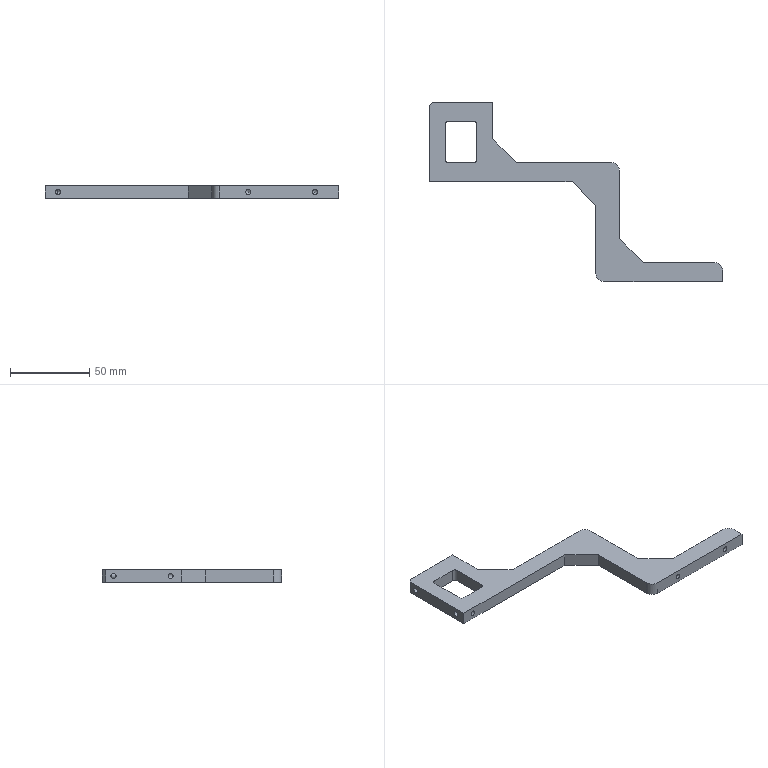Part | STEP file | SynoNew-0304-029 | 1 solid | 40 faces | box 185 x 113 x 8 mm | volume 35447 mm3 | plane 20 | cylinder 14 | cone 6 | commonest cylinder face diameters 3.2 x7 4 x4 10 x3
STEP:
#1=CARTESIAN_POINT('',(151.6,-80.,4.));
#2=VERTEX_POINT('',#1);
#3=CARTESIAN_POINT('',(148.4,-80.,4.));
#4=VERTEX_POINT('',#3);
#5=CARTESIAN_POINT('',(150.,-80.,4.));
#6=DIRECTION('',(0.,-1.,0.));
#7=DIRECTION('',(1.,0.,0.));
#8=AXIS2_PLACEMENT_3D('',#5,#6,#7);
#9=CIRCLE('',#8,1.6);
#10=EDGE_CURVE('',#2,#4,#9,.T.);
#11=ORIENTED_EDGE('',*,*,#10,.T.);
#12=CARTESIAN_POINT('',(150.,-79.039,4.));
#13=VERTEX_POINT('',#12);
#14=CARTESIAN_POINT('',(149.2,-79.519,4.));
#15=DIRECTION('',(0.8572,0.515,0.));
#16=VECTOR('',#15,0.8);
#17=LINE('',#14,#16);
#18=EDGE_CURVE('',#4,#13,#17,.T.);
#19=ORIENTED_EDGE('',*,*,#18,.T.);
#20=ORIENTED_EDGE('',*,*,#18,.F.);
#21=CARTESIAN_POINT('',(150.,-80.,4.));
#22=DIRECTION('',(0.,-1.,0.));
#23=DIRECTION('',(1.,0.,0.));
#24=AXIS2_PLACEMENT_3D('',#21,#22,#23);
#25=CIRCLE('',#24,1.6);
#26=EDGE_CURVE('',#4,#2,#25,.T.);
#27=ORIENTED_EDGE('',*,*,#26,.T.);
#28=EDGE_LOOP('',(#11,#19,#20,#27));
#29=FACE_OUTER_BOUND('',#28,.T.);
#30=CARTESIAN_POINT('',(150.,-79.519,4.));
#31=DIRECTION('',(0.,-1.,0.));
#32=DIRECTION('',(1.,0.,0.));
#33=AXIS2_PLACEMENT_3D('',#30,#31,#32);
#34=CONICAL_SURFACE('',#33,0.8,1.03);
#35=ADVANCED_FACE('',(#29),#34,.F.);
#36=CARTESIAN_POINT('',(151.6,-88.,4.));
#37=VERTEX_POINT('',#36);
#38=CARTESIAN_POINT('',(148.4,-88.,4.));
#39=VERTEX_POINT('',#38);
#40=CARTESIAN_POINT('',(150.,-88.,4.));
#41=DIRECTION('',(0.,1.,0.));
#42=DIRECTION('',(1.,0.,0.));
#43=AXIS2_PLACEMENT_3D('',#40,#41,#42);
#44=CIRCLE('',#43,1.6);
#45=EDGE_CURVE('',#37,#39,#44,.T.);
#46=ORIENTED_EDGE('',*,*,#45,.F.);
#47=CARTESIAN_POINT('',(150.,-88.,4.));
#48=DIRECTION('',(0.,1.,0.));
#49=DIRECTION('',(1.,0.,0.));
#50=AXIS2_PLACEMENT_3D('',#47,#48,#49);
#51=CIRCLE('',#50,1.6);
#52=EDGE_CURVE('',#39,#37,#51,.T.);
#53=ORIENTED_EDGE('',*,*,#52,.F.);
#54=CARTESIAN_POINT('',(148.4,-84.,4.));
#55=DIRECTION('',(0.,1.,0.));
#56=VECTOR('',#55,1.6);
#57=LINE('',#54,#56);
#58=EDGE_CURVE('',#39,#4,#57,.T.);
#59=ORIENTED_EDGE('',*,*,#58,.T.);
#60=ORIENTED_EDGE('',*,*,#10,.F.);
#61=ORIENTED_EDGE('',*,*,#26,.F.);
#62=ORIENTED_EDGE('',*,*,#58,.F.);
#63=EDGE_LOOP('',(#46,#53,#59,#60,#61,#62));
#64=FACE_OUTER_BOUND('',#63,.T.);
#65=CARTESIAN_POINT('',(150.,-84.,4.));
#66=DIRECTION('',(0.,-1.,0.));
#67=DIRECTION('',(1.,0.,0.));
#68=AXIS2_PLACEMENT_3D('',#65,#66,#67);
#69=CYLINDRICAL_SURFACE('',#68,1.6);
#70=ADVANCED_FACE('',(#64),#69,.F.);
#71=CARTESIAN_POINT('',(109.6,-80.,4.));
#72=VERTEX_POINT('',#71);
#73=CARTESIAN_POINT('',(106.4,-80.,4.));
#74=VERTEX_POINT('',#73);
#75=CARTESIAN_POINT('',(108.,-80.,4.));
#76=DIRECTION('',(0.,-1.,0.));
#77=DIRECTION('',(1.,0.,0.));
#78=AXIS2_PLACEMENT_3D('',#75,#76,#77);
#79=CIRCLE('',#78,1.6);
#80=EDGE_CURVE('',#72,#74,#79,.T.);
#81=ORIENTED_EDGE('',*,*,#80,.T.);
#82=CARTESIAN_POINT('',(108.,-79.039,4.));
#83=VERTEX_POINT('',#82);
#84=CARTESIAN_POINT('',(107.2,-79.519,4.));
#85=DIRECTION('',(0.8572,0.515,0.));
#86=VECTOR('',#85,0.8);
#87=LINE('',#84,#86);
#88=EDGE_CURVE('',#74,#83,#87,.T.);
#89=ORIENTED_EDGE('',*,*,#88,.T.);
#90=ORIENTED_EDGE('',*,*,#88,.F.);
#91=CARTESIAN_POINT('',(108.,-80.,4.));
#92=DIRECTION('',(0.,-1.,0.));
#93=DIRECTION('',(1.,0.,0.));
#94=AXIS2_PLACEMENT_3D('',#91,#92,#93);
#95=CIRCLE('',#94,1.6);
#96=EDGE_CURVE('',#74,#72,#95,.T.);
#97=ORIENTED_EDGE('',*,*,#96,.T.);
#98=EDGE_LOOP('',(#81,#89,#90,#97));
#99=FACE_OUTER_BOUND('',#98,.T.);
#100=CARTESIAN_POINT('',(108.,-79.519,4.));
#101=DIRECTION('',(0.,-1.,0.));
#102=DIRECTION('',(1.,0.,0.));
#103=AXIS2_PLACEMENT_3D('',#100,#101,#102);
#104=CONICAL_SURFACE('',#103,0.8,1.03);
#105=ADVANCED_FACE('',(#99),#104,.F.);
#106=CARTESIAN_POINT('',(109.6,-88.,4.));
#107=VERTEX_POINT('',#106);
#108=CARTESIAN_POINT('',(106.4,-88.,4.));
#109=VERTEX_POINT('',#108);
#110=CARTESIAN_POINT('',(108.,-88.,4.));
#111=DIRECTION('',(0.,1.,0.));
#112=DIRECTION('',(1.,0.,0.));
#113=AXIS2_PLACEMENT_3D('',#110,#111,#112);
#114=CIRCLE('',#113,1.6);
#115=EDGE_CURVE('',#107,#109,#114,.T.);
#116=ORIENTED_EDGE('',*,*,#115,.F.);
#117=CARTESIAN_POINT('',(108.,-88.,4.));
#118=DIRECTION('',(0.,1.,0.));
#119=DIRECTION('',(1.,0.,0.));
#120=AXIS2_PLACEMENT_3D('',#117,#118,#119);
#121=CIRCLE('',#120,1.6);
#122=EDGE_CURVE('',#109,#107,#121,.T.);
#123=ORIENTED_EDGE('',*,*,#122,.F.);
#124=CARTESIAN_POINT('',(106.4,-84.,4.));
#125=DIRECTION('',(0.,1.,0.));
#126=VECTOR('',#125,1.6);
#127=LINE('',#124,#126);
#128=EDGE_CURVE('',#109,#74,#127,.T.);
#129=ORIENTED_EDGE('',*,*,#128,.T.);
#130=ORIENTED_EDGE('',*,*,#80,.F.);
#131=ORIENTED_EDGE('',*,*,#96,.F.);
#132=ORIENTED_EDGE('',*,*,#128,.F.);
#133=EDGE_LOOP('',(#116,#123,#129,#130,#131,#132));
#134=FACE_OUTER_BOUND('',#133,.T.);
#135=CARTESIAN_POINT('',(108.,-84.,4.));
#136=DIRECTION('',(0.,-1.,0.));
#137=DIRECTION('',(1.,0.,0.));
#138=AXIS2_PLACEMENT_3D('',#135,#136,#137);
#139=CYLINDRICAL_SURFACE('',#138,1.6);
#140=ADVANCED_FACE('',(#134),#139,.F.);
#141=CARTESIAN_POINT('',(85.,-83.,0.));
#142=VERTEX_POINT('',#141);
#143=CARTESIAN_POINT('',(90.,-88.,0.));
#144=VERTEX_POINT('',#143);
#145=CARTESIAN_POINT('',(90.,-83.,0.));
#146=DIRECTION('',(0.,0.,1.));
#147=DIRECTION('',(-0.7071,-0.7071,0.));
#148=AXIS2_PLACEMENT_3D('',#145,#146,#147);
#149=CIRCLE('',#148,5.);
#150=EDGE_CURVE('',#142,#144,#149,.T.);
#151=ORIENTED_EDGE('',*,*,#150,.T.);
#152=CARTESIAN_POINT('',(90.,-88.,8.));
#153=VERTEX_POINT('',#152);
#154=CARTESIAN_POINT('',(90.,-88.,6.));
#155=DIRECTION('',(0.,0.,1.));
#156=VECTOR('',#155,10.);
#157=LINE('',#154,#156);
#158=EDGE_CURVE('',#144,#153,#157,.T.);
#159=ORIENTED_EDGE('',*,*,#158,.T.);
#160=CARTESIAN_POINT('',(85.,-83.,8.));
#161=VERTEX_POINT('',#160);
#162=CARTESIAN_POINT('',(90.,-83.,8.));
#163=DIRECTION('',(0.,0.,-1.));
#164=DIRECTION('',(-0.7071,-0.7071,0.));
#165=AXIS2_PLACEMENT_3D('',#162,#163,#164);
#166=CIRCLE('',#165,5.);
#167=EDGE_CURVE('',#153,#161,#166,.T.);
#168=ORIENTED_EDGE('',*,*,#167,.T.);
#169=CARTESIAN_POINT('',(85.,-83.,6.));
#170=DIRECTION('',(0.,0.,-1.));
#171=VECTOR('',#170,10.);
#172=LINE('',#169,#171);
#173=EDGE_CURVE('',#161,#142,#172,.T.);
#174=ORIENTED_EDGE('',*,*,#173,.T.);
#175=EDGE_LOOP('',(#151,#159,#168,#174));
#176=FACE_OUTER_BOUND('',#175,.T.);
#177=CARTESIAN_POINT('',(90.,-83.,6.));
#178=DIRECTION('',(0.,0.,-1.));
#179=DIRECTION('',(-0.7071,-0.7071,0.));
#180=AXIS2_PLACEMENT_3D('',#177,#178,#179);
#181=CYLINDRICAL_SURFACE('',#180,5.);
#182=ADVANCED_FACE('',(#176),#181,.T.);
#183=ORIENTED_EDGE('',*,*,#158,.F.);
#184=CARTESIAN_POINT('',(165.,-88.,0.));
#185=VERTEX_POINT('',#184);
#186=CARTESIAN_POINT('',(-20.,-88.,0.));
#187=DIRECTION('',(1.,0.,0.));
#188=VECTOR('',#187,10.);
#189=LINE('',#186,#188);
#190=EDGE_CURVE('',#144,#185,#189,.T.);
#191=ORIENTED_EDGE('',*,*,#190,.T.);
#192=CARTESIAN_POINT('',(165.,-88.,8.));
#193=VERTEX_POINT('',#192);
#194=CARTESIAN_POINT('',(165.,-88.,8.));
#195=DIRECTION('',(0.,0.,-1.));
#196=VECTOR('',#195,10.);
#197=LINE('',#194,#196);
#198=EDGE_CURVE('',#193,#185,#197,.T.);
#199=ORIENTED_EDGE('',*,*,#198,.F.);
#200=CARTESIAN_POINT('',(100.,-88.,8.));
#201=DIRECTION('',(1.,0.,0.));
#202=VECTOR('',#201,10.);
#203=LINE('',#200,#202);
#204=EDGE_CURVE('',#153,#193,#203,.T.);
#205=ORIENTED_EDGE('',*,*,#204,.F.);
#206=EDGE_LOOP('',(#183,#191,#199,#205));
#207=FACE_OUTER_BOUND('',#206,.T.);
#208=ORIENTED_EDGE('',*,*,#45,.T.);
#209=ORIENTED_EDGE('',*,*,#52,.T.);
#210=EDGE_LOOP('',(#208,#209));
#211=FACE_BOUND('',#210,.T.);
#212=ORIENTED_EDGE('',*,*,#115,.T.);
#213=ORIENTED_EDGE('',*,*,#122,.T.);
#214=EDGE_LOOP('',(#212,#213));
#215=FACE_BOUND('',#214,.T.);
#216=CARTESIAN_POINT('',(92.5,-88.,4.));
#217=DIRECTION('',(0.,-1.,0.));
#218=DIRECTION('',(0.,0.,-1.));
#219=AXIS2_PLACEMENT_3D('',#216,#217,#218);
#220=PLANE('',#219);
#221=ADVANCED_FACE('',(#207,#211,#215),#220,.T.);
#222=ORIENTED_EDGE('',*,*,#150,.F.);
#223=CARTESIAN_POINT('',(85.,-40.,0.));
#224=VERTEX_POINT('',#223);
#225=CARTESIAN_POINT('',(85.,-25.,0.));
#226=DIRECTION('',(0.,-1.,0.));
#227=VECTOR('',#226,10.);
#228=LINE('',#225,#227);
#229=EDGE_CURVE('',#224,#142,#228,.T.);
#230=ORIENTED_EDGE('',*,*,#229,.F.);
#231=CARTESIAN_POINT('',(70.,-25.,0.));
#232=VERTEX_POINT('',#231);
#233=CARTESIAN_POINT('',(50.,-5.,0.));
#234=DIRECTION('',(0.7071,-0.7071,0.));
#235=VECTOR('',#234,10.);
#236=LINE('',#233,#235);
#237=EDGE_CURVE('',#232,#224,#236,.T.);
#238=ORIENTED_EDGE('',*,*,#237,.F.);
#239=CARTESIAN_POINT('',(-20.,-25.,0.));
#240=VERTEX_POINT('',#239);
#241=CARTESIAN_POINT('',(-20.,-25.,0.));
#242=DIRECTION('',(1.,0.,0.));
#243=VECTOR('',#242,10.);
#244=LINE('',#241,#243);
#245=EDGE_CURVE('',#240,#232,#244,.T.);
#246=ORIENTED_EDGE('',*,*,#245,.F.);
#247=CARTESIAN_POINT('',(-20.,23.,0.));
#248=VERTEX_POINT('',#247);
#249=CARTESIAN_POINT('',(-20.,25.,0.));
#250=DIRECTION('',(0.,-1.,0.));
#251=VECTOR('',#250,10.);
#252=LINE('',#249,#251);
#253=EDGE_CURVE('',#248,#240,#252,.T.);
#254=ORIENTED_EDGE('',*,*,#253,.F.);
#255=CARTESIAN_POINT('',(-18.,25.,0.));
#256=VERTEX_POINT('',#255);
#257=CARTESIAN_POINT('',(-20.25,22.75,0.));
#258=DIRECTION('',(-0.7071,-0.7071,0.));
#259=VECTOR('',#258,10.);
#260=LINE('',#257,#259);
#261=EDGE_CURVE('',#256,#248,#260,.T.);
#262=ORIENTED_EDGE('',*,*,#261,.F.);
#263=CARTESIAN_POINT('',(20.,25.,0.));
#264=VERTEX_POINT('',#263);
#265=CARTESIAN_POINT('',(20.,25.,0.));
#266=DIRECTION('',(-1.,0.,0.));
#267=VECTOR('',#266,10.);
#268=LINE('',#265,#267);
#269=EDGE_CURVE('',#264,#256,#268,.T.);
#270=ORIENTED_EDGE('',*,*,#269,.F.);
#271=CARTESIAN_POINT('',(20.,2.,0.));
#272=VERTEX_POINT('',#271);
#273=CARTESIAN_POINT('',(20.,-25.,0.));
#274=DIRECTION('',(0.,1.,0.));
#275=VECTOR('',#274,10.);
#276=LINE('',#273,#275);
#277=EDGE_CURVE('',#272,#264,#276,.T.);
#278=ORIENTED_EDGE('',*,*,#277,.F.);
#279=CARTESIAN_POINT('',(35.,-13.,0.));
#280=VERTEX_POINT('',#279);
#281=CARTESIAN_POINT('',(19.25,2.75,0.));
#282=DIRECTION('',(-0.7071,0.7071,0.));
#283=VECTOR('',#282,10.);
#284=LINE('',#281,#283);
#285=EDGE_CURVE('',#280,#272,#284,.T.);
#286=ORIENTED_EDGE('',*,*,#285,.F.);
#287=CARTESIAN_POINT('',(95.,-13.,0.));
#288=VERTEX_POINT('',#287);
#289=CARTESIAN_POINT('',(20.,-13.,0.));
#290=DIRECTION('',(1.,0.,0.));
#291=VECTOR('',#290,10.);
#292=LINE('',#289,#291);
#293=EDGE_CURVE('',#280,#288,#292,.T.);
#294=ORIENTED_EDGE('',*,*,#293,.T.);
#295=CARTESIAN_POINT('',(100.,-18.,0.));
#296=VERTEX_POINT('',#295);
#297=CARTESIAN_POINT('',(95.,-18.,0.));
#298=DIRECTION('',(0.,0.,1.));
#299=DIRECTION('',(0.7071,0.7071,0.));
#300=AXIS2_PLACEMENT_3D('',#297,#298,#299);
#301=CIRCLE('',#300,5.);
#302=EDGE_CURVE('',#296,#288,#301,.T.);
#303=ORIENTED_EDGE('',*,*,#302,.F.);
#304=CARTESIAN_POINT('',(100.,-61.,0.));
#305=VERTEX_POINT('',#304);
#306=CARTESIAN_POINT('',(100.,-25.,0.));
#307=DIRECTION('',(0.,-1.,0.));
#308=VECTOR('',#307,10.);
#309=LINE('',#306,#308);
#310=EDGE_CURVE('',#296,#305,#309,.T.);
#311=ORIENTED_EDGE('',*,*,#310,.T.);
#312=CARTESIAN_POINT('',(115.,-76.,0.));
#313=VERTEX_POINT('',#312);
#314=CARTESIAN_POINT('',(63.5,-24.5,0.));
#315=DIRECTION('',(-0.7071,0.7071,0.));
#316=VECTOR('',#315,10.);
#317=LINE('',#314,#316);
#318=EDGE_CURVE('',#313,#305,#317,.T.);
#319=ORIENTED_EDGE('',*,*,#318,.F.);
#320=CARTESIAN_POINT('',(160.,-76.,0.));
#321=VERTEX_POINT('',#320);
#322=CARTESIAN_POINT('',(100.,-76.,0.));
#323=DIRECTION('',(1.,0.,0.));
#324=VECTOR('',#323,10.);
#325=LINE('',#322,#324);
#326=EDGE_CURVE('',#313,#321,#325,.T.);
#327=ORIENTED_EDGE('',*,*,#326,.T.);
#328=CARTESIAN_POINT('',(165.,-81.,0.));
#329=VERTEX_POINT('',#328);
#330=CARTESIAN_POINT('',(160.,-81.,0.));
#331=DIRECTION('',(0.,0.,1.));
#332=DIRECTION('',(0.7071,0.7071,0.));
#333=AXIS2_PLACEMENT_3D('',#330,#331,#332);
#334=CIRCLE('',#333,5.);
#335=EDGE_CURVE('',#329,#321,#334,.T.);
#336=ORIENTED_EDGE('',*,*,#335,.F.);
#337=CARTESIAN_POINT('',(165.,-88.,0.));
#338=DIRECTION('',(0.,1.,0.));
#339=VECTOR('',#338,10.);
#340=LINE('',#337,#339);
#341=EDGE_CURVE('',#185,#329,#340,.T.);
#342=ORIENTED_EDGE('',*,*,#341,.F.);
#343=ORIENTED_EDGE('',*,*,#190,.F.);
#344=EDGE_LOOP('',(#222,#230,#238,#246,#254,#262,#270,#278,#286,#294,#303,#311,#319,#327,#336,#342,#343));
#345=FACE_OUTER_BOUND('',#344,.T.);
#346=CARTESIAN_POINT('',(10.,-11.,0.));
#347=VERTEX_POINT('',#346);
#348=CARTESIAN_POINT('',(10.,11.,0.));
#349=VERTEX_POINT('',#348);
#350=CARTESIAN_POINT('',(10.,-6.5,0.));
#351=DIRECTION('',(0.,1.,0.));
#352=VECTOR('',#351,10.);
#353=LINE('',#350,#352);
#354=EDGE_CURVE('',#347,#349,#353,.T.);
#355=ORIENTED_EDGE('',*,*,#354,.T.);
#356=CARTESIAN_POINT('',(8.,13.,0.));
#357=VERTEX_POINT('',#356);
#358=CARTESIAN_POINT('',(8.,11.,0.));
#359=DIRECTION('',(0.,0.,-1.));
#360=DIRECTION('',(0.7071,0.7071,0.));
#361=AXIS2_PLACEMENT_3D('',#358,#359,#360);
#362=CIRCLE('',#361,2.);
#363=EDGE_CURVE('',#357,#349,#362,.T.);
#364=ORIENTED_EDGE('',*,*,#363,.F.);
#365=CARTESIAN_POINT('',(-8.,13.,0.));
#366=VERTEX_POINT('',#365);
#367=CARTESIAN_POINT('',(5.,13.,0.));
#368=DIRECTION('',(-1.,0.,0.));
#369=VECTOR('',#368,10.);
#370=LINE('',#367,#369);
#371=EDGE_CURVE('',#357,#366,#370,.T.);
#372=ORIENTED_EDGE('',*,*,#371,.T.);
#373=CARTESIAN_POINT('',(-10.,11.,0.));
#374=VERTEX_POINT('',#373);
#375=CARTESIAN_POINT('',(-8.,11.,0.));
#376=DIRECTION('',(0.,0.,-1.));
#377=DIRECTION('',(-0.7071,0.7071,0.));
#378=AXIS2_PLACEMENT_3D('',#375,#376,#377);
#379=CIRCLE('',#378,2.);
#380=EDGE_CURVE('',#374,#366,#379,.T.);
#381=ORIENTED_EDGE('',*,*,#380,.F.);
#382=CARTESIAN_POINT('',(-10.,-11.,0.));
#383=VERTEX_POINT('',#382);
#384=CARTESIAN_POINT('',(-10.,6.5,0.));
#385=DIRECTION('',(0.,-1.,0.));
#386=VECTOR('',#385,10.);
#387=LINE('',#384,#386);
#388=EDGE_CURVE('',#374,#383,#387,.T.);
#389=ORIENTED_EDGE('',*,*,#388,.T.);
#390=CARTESIAN_POINT('',(-8.,-13.,0.));
#391=VERTEX_POINT('',#390);
#392=CARTESIAN_POINT('',(-8.,-11.,0.));
#393=DIRECTION('',(0.,0.,-1.));
#394=DIRECTION('',(-0.7071,-0.7071,0.));
#395=AXIS2_PLACEMENT_3D('',#392,#393,#394);
#396=CIRCLE('',#395,2.);
#397=EDGE_CURVE('',#391,#383,#396,.T.);
#398=ORIENTED_EDGE('',*,*,#397,.F.);
#399=CARTESIAN_POINT('',(8.,-13.,0.));
#400=VERTEX_POINT('',#399);
#401=CARTESIAN_POINT('',(-5.,-13.,0.));
#402=DIRECTION('',(1.,0.,0.));
#403=VECTOR('',#402,10.);
#404=LINE('',#401,#403);
#405=EDGE_CURVE('',#391,#400,#404,.T.);
#406=ORIENTED_EDGE('',*,*,#405,.T.);
#407=CARTESIAN_POINT('',(8.,-11.,0.));
#408=DIRECTION('',(0.,0.,-1.));
#409=DIRECTION('',(0.7071,-0.7071,0.));
#410=AXIS2_PLACEMENT_3D('',#407,#408,#409);
#411=CIRCLE('',#410,2.);
#412=EDGE_CURVE('',#347,#400,#411,.T.);
#413=ORIENTED_EDGE('',*,*,#412,.F.);
#414=EDGE_LOOP('',(#355,#364,#372,#381,#389,#398,#406,#413));
#415=FACE_BOUND('',#414,.T.);
#416=CARTESIAN_POINT('',(0.,0.,0.));
#417=DIRECTION('',(0.,0.,1.));
#418=DIRECTION('',(1.,0.,0.));
#419=AXIS2_PLACEMENT_3D('',#416,#417,#418);
#420=PLANE('',#419);
#421=ADVANCED_FACE('',(#345,#415),#420,.F.);
#422=CARTESIAN_POINT('',(160.,-76.,8.));
#423=VERTEX_POINT('',#422);
#424=CARTESIAN_POINT('',(165.,-81.,8.));
#425=VERTEX_POINT('',#424);
#426=CARTESIAN_POINT('',(160.,-81.,8.));
#427=DIRECTION('',(0.,0.,-1.));
#428=DIRECTION('',(0.7071,0.7071,0.));
#429=AXIS2_PLACEMENT_3D('',#426,#427,#428);
#430=CIRCLE('',#429,5.);
#431=EDGE_CURVE('',#423,#425,#430,.T.);
#432=ORIENTED_EDGE('',*,*,#431,.T.);
#433=CARTESIAN_POINT('',(165.,-81.,2.));
#434=DIRECTION('',(0.,0.,-1.));
#435=VECTOR('',#434,10.);
#436=LINE('',#433,#435);
#437=EDGE_CURVE('',#425,#329,#436,.T.);
#438=ORIENTED_EDGE('',*,*,#437,.T.);
#439=ORIENTED_EDGE('',*,*,#335,.T.);
#440=CARTESIAN_POINT('',(160.,-76.,2.));
#441=DIRECTION('',(0.,0.,1.));
#442=VECTOR('',#441,10.);
#443=LINE('',#440,#442);
#444=EDGE_CURVE('',#321,#423,#443,.T.);
#445=ORIENTED_EDGE('',*,*,#444,.T.);
#446=EDGE_LOOP('',(#432,#438,#439,#445));
#447=FACE_OUTER_BOUND('',#446,.T.);
#448=CARTESIAN_POINT('',(160.,-81.,2.));
#449=DIRECTION('',(0.,0.,1.));
#450=DIRECTION('',(0.7071,0.7071,0.));
#451=AXIS2_PLACEMENT_3D('',#448,#449,#450);
#452=CYLINDRICAL_SURFACE('',#451,5.);
#453=ADVANCED_FACE('',(#447),#452,.T.);
#454=ORIENTED_EDGE('',*,*,#444,.F.);
#455=ORIENTED_EDGE('',*,*,#326,.F.);
#456=CARTESIAN_POINT('',(115.,-76.,8.));
#457=VERTEX_POINT('',#456);
#458=CARTESIAN_POINT('',(115.,-76.,2.));
#459=DIRECTION('',(0.,0.,-1.));
#460=VECTOR('',#459,10.);
#461=LINE('',#458,#460);
#462=EDGE_CURVE('',#457,#313,#461,.T.);
#463=ORIENTED_EDGE('',*,*,#462,.F.);
#464=CARTESIAN_POINT('',(100.,-76.,8.));
#465=DIRECTION('',(1.,0.,0.));
#466=VECTOR('',#465,10.);
#467=LINE('',#464,#466);
#468=EDGE_CURVE('',#457,#423,#467,.T.);
#469=ORIENTED_EDGE('',*,*,#468,.T.);
#470=EDGE_LOOP('',(#454,#455,#463,#469));
#471=FACE_OUTER_BOUND('',#470,.T.);
#472=CARTESIAN_POINT('',(100.,-76.,0.));
#473=DIRECTION('',(0.,1.,0.));
#474=DIRECTION('',(0.,0.,1.));
#475=AXIS2_PLACEMENT_3D('',#472,#473,#474);
#476=PLANE('',#475);
#477=ADVANCED_FACE('',(#471),#476,.T.);
#478=CARTESIAN_POINT('',(95.,-13.,8.));
#479=VERTEX_POINT('',#478);
#480=CARTESIAN_POINT('',(100.,-18.,8.));
#481=VERTEX_POINT('',#480);
#482=CARTESIAN_POINT('',(95.,-18.,8.));
#483=DIRECTION('',(0.,0.,-1.));
#484=DIRECTION('',(0.7071,0.7071,0.));
#485=AXIS2_PLACEMENT_3D('',#482,#483,#484);
#486=CIRCLE('',#485,5.);
#487=EDGE_CURVE('',#479,#481,#486,.T.);
#488=ORIENTED_EDGE('',*,*,#487,.T.);
#489=CARTESIAN_POINT('',(100.,-18.,2.));
#490=DIRECTION('',(0.,0.,-1.));
#491=VECTOR('',#490,10.);
#492=LINE('',#489,#491);
#493=EDGE_CURVE('',#481,#296,#492,.T.);
#494=ORIENTED_EDGE('',*,*,#493,.T.);
#495=ORIENTED_EDGE('',*,*,#302,.T.);
#496=CARTESIAN_POINT('',(95.,-13.,2.));
#497=DIRECTION('',(0.,0.,1.));
#498=VECTOR('',#497,10.);
#499=LINE('',#496,#498);
#500=EDGE_CURVE('',#288,#479,#499,.T.);
#501=ORIENTED_EDGE('',*,*,#500,.T.);
#502=EDGE_LOOP('',(#488,#494,#495,#501));
#503=FACE_OUTER_BOUND('',#502,.T.);
#504=CARTESIAN_POINT('',(95.,-18.,2.));
#505=DIRECTION('',(0.,0.,1.));
#506=DIRECTION('',(0.7071,0.7071,0.));
#507=AXIS2_PLACEMENT_3D('',#504,#505,#506);
#508=CYLINDRICAL_SURFACE('',#507,5.);
#509=ADVANCED_FACE('',(#503),#508,.T.);
#510=ORIENTED_EDGE('',*,*,#493,.F.);
#511=CARTESIAN_POINT('',(100.,-61.,8.));
#512=VERTEX_POINT('',#511);
#513=CARTESIAN_POINT('',(100.,25.,8.));
#514=DIRECTION('',(0.,-1.,0.));
#515=VECTOR('',#514,10.);
#516=LINE('',#513,#515);
#517=EDGE_CURVE('',#481,#512,#516,.T.);
#518=ORIENTED_EDGE('',*,*,#517,.T.);
#519=CARTESIAN_POINT('',(100.,-61.,2.));
#520=DIRECTION('',(0.,0.,1.));
#521=VECTOR('',#520,10.);
#522=LINE('',#519,#521);
#523=EDGE_CURVE('',#305,#512,#522,.T.);
#524=ORIENTED_EDGE('',*,*,#523,.F.);
#525=ORIENTED_EDGE('',*,*,#310,.F.);
#526=EDGE_LOOP('',(#510,#518,#524,#525));
#527=FACE_OUTER_BOUND('',#526,.T.);
#528=CARTESIAN_POINT('',(100.,-19.,4.));
#529=DIRECTION('',(1.,0.,0.));
#530=DIRECTION('',(0.,0.,-1.));
#531=AXIS2_PLACEMENT_3D('',#528,#529,#530);
#532=PLANE('',#531);
#533=ADVANCED_FACE('',(#527),#532,.T.);
#534=ORIENTED_EDGE('',*,*,#380,.T.);
#535=CARTESIAN_POINT('',(-8.,13.,8.));
#536=VERTEX_POINT('',#535);
#537=CARTESIAN_POINT('',(-8.,13.,0.));
#538=DIRECTION('',(0.,0.,1.));
#539=VECTOR('',#538,10.);
#540=LINE('',#537,#539);
#541=EDGE_CURVE('',#366,#536,#540,.T.);
#542=ORIENTED_EDGE('',*,*,#541,.T.);
#543=CARTESIAN_POINT('',(-10.,11.,8.));
#544=VERTEX_POINT('',#543);
#545=CARTESIAN_POINT('',(-8.,11.,8.));
#546=DIRECTION('',(0.,0.,1.));
#547=DIRECTION('',(-0.7071,0.7071,0.));
#548=AXIS2_PLACEMENT_3D('',#545,#546,#547);
#549=CIRCLE('',#548,2.);
#550=EDGE_CURVE('',#536,#544,#549,.T.);
#551=ORIENTED_EDGE('',*,*,#550,.T.);
#552=CARTESIAN_POINT('',(-10.,11.,0.));
#553=DIRECTION('',(0.,0.,-1.));
#554=VECTOR('',#553,10.);
#555=LINE('',#552,#554);
#556=EDGE_CURVE('',#544,#374,#555,.T.);
#557=ORIENTED_EDGE('',*,*,#556,.T.);
#558=EDGE_LOOP('',(#534,#542,#551,#557));
#559=FACE_OUTER_BOUND('',#558,.T.);
#560=CARTESIAN_POINT('',(-8.,11.,0.));
#561=DIRECTION('',(0.,0.,1.));
#562=DIRECTION('',(-0.7071,0.7071,0.));
#563=AXIS2_PLACEMENT_3D('',#560,#561,#562);
#564=CYLINDRICAL_SURFACE('',#563,2.);
#565=ADVANCED_FACE('',(#559),#564,.F.);
#566=ORIENTED_EDGE('',*,*,#541,.F.);
#567=ORIENTED_EDGE('',*,*,#371,.F.);
#568=CARTESIAN_POINT('',(8.,13.,8.));
#569=VERTEX_POINT('',#568);
#570=CARTESIAN_POINT('',(8.,13.,0.));
#571=DIRECTION('',(0.,0.,-1.));
#572=VECTOR('',#571,10.);
#573=LINE('',#570,#572);
#574=EDGE_CURVE('',#569,#357,#573,.T.);
#575=ORIENTED_EDGE('',*,*,#574,.F.);
#576=CARTESIAN_POINT('',(5.,13.,8.));
#577=DIRECTION('',(1.,0.,0.));
#578=VECTOR('',#577,10.);
#579=LINE('',#576,#578);
#580=EDGE_CURVE('',#536,#569,#579,.T.);
#581=ORIENTED_EDGE('',*,*,#580,.F.);
#582=EDGE_LOOP('',(#566,#567,#575,#581));
#583=FACE_OUTER_BOUND('',#582,.T.);
#584=CARTESIAN_POINT('',(10.,13.,0.));
#585=DIRECTION('',(0.,1.,0.));
#586=DIRECTION('',(-1.,0.,0.));
#587=AXIS2_PLACEMENT_3D('',#584,#585,#586);
#588=PLANE('',#587);
#589=ADVANCED_FACE('',(#583),#588,.F.);
#590=ORIENTED_EDGE('',*,*,#363,.T.);
#591=CARTESIAN_POINT('',(10.,11.,8.));
#592=VERTEX_POINT('',#591);
#593=CARTESIAN_POINT('',(10.,11.,0.));
#594=DIRECTION('',(0.,0.,1.));
#595=VECTOR('',#594,10.);
#596=LINE('',#593,#595);
#597=EDGE_CURVE('',#349,#592,#596,.T.);
#598=ORIENTED_EDGE('',*,*,#597,.T.);
#599=CARTESIAN_POINT('',(8.,11.,8.));
#600=DIRECTION('',(0.,0.,1.));
#601=DIRECTION('',(0.7071,0.7071,0.));
#602=AXIS2_PLACEMENT_3D('',#599,#600,#601);
#603=CIRCLE('',#602,2.);
#604=EDGE_CURVE('',#592,#569,#603,.T.);
#605=ORIENTED_EDGE('',*,*,#604,.T.);
#606=ORIENTED_EDGE('',*,*,#574,.T.);
#607=EDGE_LOOP('',(#590,#598,#605,#606));
#608=FACE_OUTER_BOUND('',#607,.T.);
#609=CARTESIAN_POINT('',(8.,11.,0.));
#610=DIRECTION('',(0.,0.,1.));
#611=DIRECTION('',(0.7071,0.7071,0.));
#612=AXIS2_PLACEMENT_3D('',#609,#610,#611);
#613=CYLINDRICAL_SURFACE('',#612,2.);
#614=ADVANCED_FACE('',(#608),#613,.F.);
#615=ORIENTED_EDGE('',*,*,#597,.F.);
#616=ORIENTED_EDGE('',*,*,#354,.F.);
#617=CARTESIAN_POINT('',(10.,-11.,8.));
#618=VERTEX_POINT('',#617);
#619=CARTESIAN_POINT('',(10.,-11.,0.));
#620=DIRECTION('',(0.,0.,-1.));
#621=VECTOR('',#620,10.);
#622=LINE('',#619,#621);
#623=EDGE_CURVE('',#618,#347,#622,.T.);
#624=ORIENTED_EDGE('',*,*,#623,.F.);
#625=CARTESIAN_POINT('',(10.,-6.5,8.));
#626=DIRECTION('',(0.,-1.,0.));
#627=VECTOR('',#626,10.);
#628=LINE('',#625,#627);
#629=EDGE_CURVE('',#592,#618,#628,.T.);
#630=ORIENTED_EDGE('',*,*,#629,.F.);
#631=EDGE_LOOP('',(#615,#616,#624,#630));
#632=FACE_OUTER_BOUND('',#631,.T.);
#633=CARTESIAN_POINT('',(10.,-13.,0.));
#634=DIRECTION('',(1.,0.,0.));
#635=DIRECTION('',(0.,1.,0.));
#636=AXIS2_PLACEMENT_3D('',#633,#634,#635);
#637=PLANE('',#636);
#638=ADVANCED_FACE('',(#632),#637,.F.);
#639=ORIENTED_EDGE('',*,*,#412,.T.);
#640=CARTESIAN_POINT('',(8.,-13.,8.));
#641=VERTEX_POINT('',#640);
#642=CARTESIAN_POINT('',(8.,-13.,0.));
#643=DIRECTION('',(0.,0.,1.));
#644=VECTOR('',#643,10.);
#645=LINE('',#642,#644);
#646=EDGE_CURVE('',#400,#641,#645,.T.);
#647=ORIENTED_EDGE('',*,*,#646,.T.);
#648=CARTESIAN_POINT('',(8.,-11.,8.));
#649=DIRECTION('',(0.,0.,1.));
#650=DIRECTION('',(0.7071,-0.7071,0.));
#651=AXIS2_PLACEMENT_3D('',#648,#649,#650);
#652=CIRCLE('',#651,2.);
#653=EDGE_CURVE('',#641,#618,#652,.T.);
#654=ORIENTED_EDGE('',*,*,#653,.T.);
#655=ORIENTED_EDGE('',*,*,#623,.T.);
#656=EDGE_LOOP('',(#639,#647,#654,#655));
#657=FACE_OUTER_BOUND('',#656,.T.);
#658=CARTESIAN_POINT('',(8.,-11.,0.));
#659=DIRECTION('',(0.,0.,1.));
#660=DIRECTION('',(0.7071,-0.7071,0.));
#661=AXIS2_PLACEMENT_3D('',#658,#659,#660);
#662=CYLINDRICAL_SURFACE('',#661,2.);
#663=ADVANCED_FACE('',(#657),#662,.F.);
#664=ORIENTED_EDGE('',*,*,#646,.F.);
#665=ORIENTED_EDGE('',*,*,#405,.F.);
#666=CARTESIAN_POINT('',(-8.,-13.,8.));
#667=VERTEX_POINT('',#666);
#668=CARTESIAN_POINT('',(-8.,-13.,0.));
#669=DIRECTION('',(0.,0.,-1.));
#670=VECTOR('',#669,10.);
#671=LINE('',#668,#670);
#672=EDGE_CURVE('',#667,#391,#671,.T.);
#673=ORIENTED_EDGE('',*,*,#672,.F.);
#674=CARTESIAN_POINT('',(-5.,-13.,8.));
#675=DIRECTION('',(-1.,0.,0.));
#676=VECTOR('',#675,10.);
#677=LINE('',#674,#676);
#678=EDGE_CURVE('',#641,#667,#677,.T.);
#679=ORIENTED_EDGE('',*,*,#678,.F.);
#680=EDGE_LOOP('',(#664,#665,#673,#679));
#681=FACE_OUTER_BOUND('',#680,.T.);
#682=CARTESIAN_POINT('',(-10.,-13.,0.));
#683=DIRECTION('',(0.,-1.,0.));
#684=DIRECTION('',(1.,0.,0.));
#685=AXIS2_PLACEMENT_3D('',#682,#683,#684);
#686=PLANE('',#685);
#687=ADVANCED_FACE('',(#681),#686,.F.);
#688=ORIENTED_EDGE('',*,*,#397,.T.);
#689=CARTESIAN_POINT('',(-10.,-11.,8.));
#690=VERTEX_POINT('',#689);
#691=CARTESIAN_POINT('',(-10.,-11.,0.));
#692=DIRECTION('',(0.,0.,1.));
#693=VECTOR('',#692,10.);
#694=LINE('',#691,#693);
#695=EDGE_CURVE('',#383,#690,#694,.T.);
#696=ORIENTED_EDGE('',*,*,#695,.T.);
#697=CARTESIAN_POINT('',(-8.,-11.,8.));
#698=DIRECTION('',(0.,0.,1.));
#699=DIRECTION('',(-0.7071,-0.7071,0.));
#700=AXIS2_PLACEMENT_3D('',#697,#698,#699);
#701=CIRCLE('',#700,2.);
#702=EDGE_CURVE('',#690,#667,#701,.T.);
#703=ORIENTED_EDGE('',*,*,#702,.T.);
#704=ORIENTED_EDGE('',*,*,#672,.T.);
#705=EDGE_LOOP('',(#688,#696,#703,#704));
#706=FACE_OUTER_BOUND('',#705,.T.);
#707=CARTESIAN_POINT('',(-8.,-11.,0.));
#708=DIRECTION('',(0.,0.,1.));
#709=DIRECTION('',(-0.7071,-0.7071,0.));
#710=AXIS2_PLACEMENT_3D('',#707,#708,#709);
#711=CYLINDRICAL_SURFACE('',#710,2.);
#712=ADVANCED_FACE('',(#706),#711,.F.);
#713=ORIENTED_EDGE('',*,*,#556,.F.);
#714=CARTESIAN_POINT('',(-10.,6.5,8.));
#715=DIRECTION('',(0.,1.,0.));
#716=VECTOR('',#715,10.);
#717=LINE('',#714,#716);
#718=EDGE_CURVE('',#690,#544,#717,.T.);
#719=ORIENTED_EDGE('',*,*,#718,.F.);
#720=ORIENTED_EDGE('',*,*,#695,.F.);
#721=ORIENTED_EDGE('',*,*,#388,.F.);
#722=EDGE_LOOP('',(#713,#719,#720,#721));
#723=FACE_OUTER_BOUND('',#722,.T.);
#724=CARTESIAN_POINT('',(-10.,13.,0.));
#725=DIRECTION('',(-1.,0.,0.));
#726=DIRECTION('',(0.,-1.,0.));
#727=AXIS2_PLACEMENT_3D('',#724,#725,#726);
#728=PLANE('',#727);
#729=ADVANCED_FACE('',(#723),#728,.F.);
#730=CARTESIAN_POINT('',(20.,2.,8.));
#731=VERTEX_POINT('',#730);
#732=CARTESIAN_POINT('',(35.,-13.,8.));
#733=VERTEX_POINT('',#732);
#734=CARTESIAN_POINT('',(19.25,2.75,8.));
#735=DIRECTION('',(0.7071,-0.7071,0.));
#736=VECTOR('',#735,10.);
#737=LINE('',#734,#736);
#738=EDGE_CURVE('',#731,#733,#737,.T.);
#739=ORIENTED_EDGE('',*,*,#738,.T.);
#740=CARTESIAN_POINT('',(35.,-13.,0.));
#741=DIRECTION('',(0.,0.,-1.));
#742=VECTOR('',#741,10.);
#743=LINE('',#740,#742);
#744=EDGE_CURVE('',#733,#280,#743,.T.);
#745=ORIENTED_EDGE('',*,*,#744,.T.);
#746=ORIENTED_EDGE('',*,*,#285,.T.);
#747=CARTESIAN_POINT('',(20.,2.,0.));
#748=DIRECTION('',(0.,0.,1.));
#749=VECTOR('',#748,10.);
#750=LINE('',#747,#749);
#751=EDGE_CURVE('',#272,#731,#750,.T.);
#752=ORIENTED_EDGE('',*,*,#751,.T.);
#753=EDGE_LOOP('',(#739,#745,#746,#752));
#754=FACE_OUTER_BOUND('',#753,.T.);
#755=CARTESIAN_POINT('',(27.5,-5.5,0.));
#756=DIRECTION('',(0.7071,0.7071,0.));
#757=DIRECTION('',(0.,0.,-1.));
#758=AXIS2_PLACEMENT_3D('',#755,#756,#757);
#759=PLANE('',#758);
#760=ADVANCED_FACE('',(#754),#759,.T.);
#761=ORIENTED_EDGE('',*,*,#500,.F.);
#762=ORIENTED_EDGE('',*,*,#293,.F.);
#763=ORIENTED_EDGE('',*,*,#744,.F.);
#764=CARTESIAN_POINT('',(20.,-13.,8.));
#765=DIRECTION('',(1.,0.,0.));
#766=VECTOR('',#765,10.);
#767=LINE('',#764,#766);
#768=EDGE_CURVE('',#733,#479,#767,.T.);
#769=ORIENTED_EDGE('',*,*,#768,.T.);
#770=EDGE_LOOP('',(#761,#762,#763,#769));
#771=FACE_OUTER_BOUND('',#770,.T.);
#772=CARTESIAN_POINT('',(20.,-13.,0.));
#773=DIRECTION('',(0.,1.,0.));
#774=DIRECTION('',(0.,0.,1.));
#775=AXIS2_PLACEMENT_3D('',#772,#773,#774);
#776=PLANE('',#775);
#777=ADVANCED_FACE('',(#771),#776,.T.);
#778=CARTESIAN_POINT('',(63.5,-24.5,8.));
#779=DIRECTION('',(0.7071,-0.7071,0.));
#780=VECTOR('',#779,10.);
#781=LINE('',#778,#780);
#782=EDGE_CURVE('',#512,#457,#781,.T.);
#783=ORIENTED_EDGE('',*,*,#782,.T.);
#784=ORIENTED_EDGE('',*,*,#462,.T.);
#785=ORIENTED_EDGE('',*,*,#318,.T.);
#786=ORIENTED_EDGE('',*,*,#523,.T.);
#787=EDGE_LOOP('',(#783,#784,#785,#786));
#788=FACE_OUTER_BOUND('',#787,.T.);
#789=CARTESIAN_POINT('',(107.5,-68.5,2.));
#790=DIRECTION('',(0.7071,0.7071,0.));
#791=DIRECTION('',(0.,0.,-1.));
#792=AXIS2_PLACEMENT_3D('',#789,#790,#791);
#793=PLANE('',#792);
#794=ADVANCED_FACE('',(#788),#793,.T.);
#795=ORIENTED_EDGE('',*,*,#237,.T.);
#796=CARTESIAN_POINT('',(85.,-40.,8.));
#797=VERTEX_POINT('',#796);
#798=CARTESIAN_POINT('',(85.,-40.,4.));
#799=DIRECTION('',(0.,0.,1.));
#800=VECTOR('',#799,10.);
#801=LINE('',#798,#800);
#802=EDGE_CURVE('',#224,#797,#801,.T.);
#803=ORIENTED_EDGE('',*,*,#802,.T.);
#804=CARTESIAN_POINT('',(70.,-25.,8.));
#805=VERTEX_POINT('',#804);
#806=CARTESIAN_POINT('',(50.,-5.,8.));
#807=DIRECTION('',(-0.7071,0.7071,0.));
#808=VECTOR('',#807,10.);
#809=LINE('',#806,#808);
#810=EDGE_CURVE('',#797,#805,#809,.T.);
#811=ORIENTED_EDGE('',*,*,#810,.T.);
#812=CARTESIAN_POINT('',(70.,-25.,4.));
#813=DIRECTION('',(0.,0.,-1.));
#814=VECTOR('',#813,10.);
#815=LINE('',#812,#814);
#816=EDGE_CURVE('',#805,#232,#815,.T.);
#817=ORIENTED_EDGE('',*,*,#816,.T.);
#818=EDGE_LOOP('',(#795,#803,#811,#817));
#819=FACE_OUTER_BOUND('',#818,.T.);
#820=CARTESIAN_POINT('',(77.5,-32.5,4.));
#821=DIRECTION('',(-0.7071,-0.7071,0.));
#822=DIRECTION('',(0.,0.,1.));
#823=AXIS2_PLACEMENT_3D('',#820,#821,#822);
#824=PLANE('',#823);
#825=ADVANCED_FACE('',(#819),#824,.T.);
#826=ORIENTED_EDGE('',*,*,#173,.F.);
#827=CARTESIAN_POINT('',(85.,-25.,8.));
#828=DIRECTION('',(0.,-1.,0.));
#829=VECTOR('',#828,10.);
#830=LINE('',#827,#829);
#831=EDGE_CURVE('',#797,#161,#830,.T.);
#832=ORIENTED_EDGE('',*,*,#831,.F.);
#833=ORIENTED_EDGE('',*,*,#802,.F.);
#834=ORIENTED_EDGE('',*,*,#229,.T.);
#835=EDGE_LOOP('',(#826,#832,#833,#834));
#836=FACE_OUTER_BOUND('',#835,.T.);
#837=CARTESIAN_POINT('',(85.,-25.,8.));
#838=DIRECTION('',(-1.,0.,0.));
#839=DIRECTION('',(0.,0.,-1.));
#840=AXIS2_PLACEMENT_3D('',#837,#838,#839);
#841=PLANE('',#840);
#842=ADVANCED_FACE('',(#836),#841,.T.);
#843=ORIENTED_EDGE('',*,*,#437,.F.);
#844=CARTESIAN_POINT('',(165.,-13.,8.));
#845=DIRECTION('',(0.,-1.,0.));
#846=VECTOR('',#845,10.);
#847=LINE('',#844,#846);
#848=EDGE_CURVE('',#425,#193,#847,.T.);
#849=ORIENTED_EDGE('',*,*,#848,.T.);
#850=ORIENTED_EDGE('',*,*,#198,.T.);
#851=ORIENTED_EDGE('',*,*,#341,.T.);
#852=EDGE_LOOP('',(#843,#849,#850,#851));
#853=FACE_OUTER_BOUND('',#852,.T.);
#854=CARTESIAN_POINT('',(165.,-82.,4.));
#855=DIRECTION('',(1.,0.,0.));
#856=DIRECTION('',(0.,0.,-1.));
#857=AXIS2_PLACEMENT_3D('',#854,#855,#856);
#858=PLANE('',#857);
#859=ADVANCED_FACE('',(#853),#858,.T.);
#860=ORIENTED_EDGE('',*,*,#751,.F.);
#861=ORIENTED_EDGE('',*,*,#277,.T.);
#862=CARTESIAN_POINT('',(20.,25.,8.));
#863=VERTEX_POINT('',#862);
#864=CARTESIAN_POINT('',(20.,25.,0.));
#865=DIRECTION('',(0.,0.,1.));
#866=VECTOR('',#865,10.);
#867=LINE('',#864,#866);
#868=EDGE_CURVE('',#264,#863,#867,.T.);
#869=ORIENTED_EDGE('',*,*,#868,.T.);
#870=CARTESIAN_POINT('',(20.,-25.,8.));
#871=DIRECTION('',(0.,1.,0.));
#872=VECTOR('',#871,10.);
#873=LINE('',#870,#872);
#874=EDGE_CURVE('',#731,#863,#873,.T.);
#875=ORIENTED_EDGE('',*,*,#874,.F.);
#876=EDGE_LOOP('',(#860,#861,#869,#875));
#877=FACE_OUTER_BOUND('',#876,.T.);
#878=CARTESIAN_POINT('',(20.,-25.,0.));
#879=DIRECTION('',(1.,0.,0.));
#880=DIRECTION('',(0.,1.,0.));
#881=AXIS2_PLACEMENT_3D('',#878,#879,#880);
#882=PLANE('',#881);
#883=ADVANCED_FACE('',(#877),#882,.T.);
#884=CARTESIAN_POINT('',(-13.,-17.,2.751));
#885=VERTEX_POINT('',#884);
#886=CARTESIAN_POINT('',(-12.601,-16.4,4.));
#887=VERTEX_POINT('',#886);
#888=CARTESIAN_POINT('',(-13.,-17.,2.751));
#889=CARTESIAN_POINT('',(-12.955,-16.973,2.773));
#890=CARTESIAN_POINT('',(-12.91,-16.945,2.796));
#891=CARTESIAN_POINT('',(-12.759,-16.848,2.885));
#892=CARTESIAN_POINT('',(-12.654,-16.779,2.956));
#893=CARTESIAN_POINT('',(-12.541,-16.651,3.136));
#894=CARTESIAN_POINT('',(-12.521,-16.611,3.203));
#895=CARTESIAN_POINT('',(-12.513,-16.538,3.346));
#896=CARTESIAN_POINT('',(-12.524,-16.506,3.422));
#897=CARTESIAN_POINT('',(-12.567,-16.428,3.659));
#898=CARTESIAN_POINT('',(-12.601,-16.4,3.832));
#899=CARTESIAN_POINT('',(-12.601,-16.4,4.));
#900=B_SPLINE_CURVE_WITH_KNOTS('',3,(#888,#889,#890,#891,#892,#893,#894,#895,#896,#897,#898,#899),.UNSPECIFIED.,.F.,.F.,(4,2,2,2,2,4),(-0.2703,-0.251,-0.2022,-0.1769,-0.1516,-0.1011),.UNSPECIFIED.);
#901=EDGE_CURVE('',#885,#887,#900,.T.);
#902=ORIENTED_EDGE('',*,*,#901,.F.);
#903=CARTESIAN_POINT('',(-13.,-17.,5.249));
#904=VERTEX_POINT('',#903);
#905=CARTESIAN_POINT('',(-12.,-17.,4.));
#906=DIRECTION('',(0.,-1.,0.));
#907=DIRECTION('',(1.,0.,0.));
#908=AXIS2_PLACEMENT_3D('',#905,#906,#907);
#909=CIRCLE('',#908,1.6);
#910=EDGE_CURVE('',#885,#904,#909,.T.);
#911=ORIENTED_EDGE('',*,*,#910,.T.);
#912=CARTESIAN_POINT('',(-12.601,-16.4,4.));
#913=CARTESIAN_POINT('',(-12.601,-16.4,4.168));
#914=CARTESIAN_POINT('',(-12.567,-16.428,4.341));
#915=CARTESIAN_POINT('',(-12.524,-16.506,4.578));
#916=CARTESIAN_POINT('',(-12.513,-16.538,4.654));
#917=CARTESIAN_POINT('',(-12.521,-16.611,4.797));
#918=CARTESIAN_POINT('',(-12.541,-16.651,4.864));
#919=CARTESIAN_POINT('',(-12.58,-16.695,4.925));
#920=CARTESIAN_POINT('',(-12.654,-16.779,5.044));
#921=CARTESIAN_POINT('',(-12.759,-16.848,5.115));
#922=CARTESIAN_POINT('',(-12.91,-16.945,5.204));
#923=CARTESIAN_POINT('',(-12.955,-16.973,5.227));
#924=CARTESIAN_POINT('',(-13.,-17.,5.249));
#925=B_SPLINE_CURVE_WITH_KNOTS('',3,(#912,#913,#914,#915,#916,#917,#918,#919,#920,#921,#922,#923,#924),.UNSPECIFIED.,.F.,.F.,(4,2,2,3,2,4),(-0.1011,-0.05054,-0.02527,0.,0.0488,0.06818),.UNSPECIFIED.);
#926=EDGE_CURVE('',#887,#904,#925,.T.);
#927=ORIENTED_EDGE('',*,*,#926,.F.);
#928=CARTESIAN_POINT('',(-12.,-16.039,4.));
#929=VERTEX_POINT('',#928);
#930=CARTESIAN_POINT('',(-12.8,-16.519,4.));
#931=DIRECTION('',(0.8572,0.515,0.));
#932=VECTOR('',#931,0.8);
#933=LINE('',#930,#932);
#934=EDGE_CURVE('',#887,#929,#933,.T.);
#935=ORIENTED_EDGE('',*,*,#934,.T.);
#936=ORIENTED_EDGE('',*,*,#934,.F.);
#937=EDGE_LOOP('',(#902,#911,#927,#935,#936));
#938=FACE_OUTER_BOUND('',#937,.T.);
#939=CARTESIAN_POINT('',(-12.,-16.519,4.));
#940=DIRECTION('',(0.,-1.,0.));
#941=DIRECTION('',(1.,0.,0.));
#942=AXIS2_PLACEMENT_3D('',#939,#940,#941);
#943=CONICAL_SURFACE('',#942,0.8,1.03);
#944=ADVANCED_FACE('',(#938),#943,.F.);
#945=CARTESIAN_POINT('',(-10.4,-25.,4.));
#946=VERTEX_POINT('',#945);
#947=CARTESIAN_POINT('',(-13.6,-25.,4.));
#948=VERTEX_POINT('',#947);
#949=CARTESIAN_POINT('',(-12.,-25.,4.));
#950=DIRECTION('',(0.,1.,0.));
#951=DIRECTION('',(1.,0.,0.));
#952=AXIS2_PLACEMENT_3D('',#949,#950,#951);
#953=CIRCLE('',#952,1.6);
#954=EDGE_CURVE('',#946,#948,#953,.T.);
#955=ORIENTED_EDGE('',*,*,#954,.F.);
#956=CARTESIAN_POINT('',(-12.,-25.,4.));
#957=DIRECTION('',(0.,1.,0.));
#958=DIRECTION('',(1.,0.,0.));
#959=AXIS2_PLACEMENT_3D('',#956,#957,#958);
#960=CIRCLE('',#959,1.6);
#961=EDGE_CURVE('',#948,#946,#960,.T.);
#962=ORIENTED_EDGE('',*,*,#961,.F.);
#963=CARTESIAN_POINT('',(-13.6,-19.6,4.));
#964=VERTEX_POINT('',#963);
#965=CARTESIAN_POINT('',(-13.6,-21.,4.));
#966=DIRECTION('',(0.,1.,0.));
#967=VECTOR('',#966,1.6);
#968=LINE('',#965,#967);
#969=EDGE_CURVE('',#948,#964,#968,.T.);
#970=ORIENTED_EDGE('',*,*,#969,.T.);
#971=CARTESIAN_POINT('',(-12.,-18.,5.6));
#972=VERTEX_POINT('',#971);
#973=CARTESIAN_POINT('',(-12.,-18.,4.));
#974=DIRECTION('',(0.7071,-0.7071,0.));
#975=DIRECTION('',(0.7071,0.7071,0.));
#976=AXIS2_PLACEMENT_3D('',#973,#974,#975);
#977=ELLIPSE('',#976,2.263,1.6);
#978=EDGE_CURVE('',#972,#964,#977,.T.);
#979=ORIENTED_EDGE('',*,*,#978,.F.);
#980=CARTESIAN_POINT('',(-12.,-18.,4.));
#981=DIRECTION('',(0.7071,0.7071,0.));
#982=DIRECTION('',(0.7071,-0.7071,0.));
#983=AXIS2_PLACEMENT_3D('',#980,#981,#982);
#984=ELLIPSE('',#983,2.263,1.6);
#985=EDGE_CURVE('',#904,#972,#984,.T.);
#986=ORIENTED_EDGE('',*,*,#985,.F.);
#987=ORIENTED_EDGE('',*,*,#910,.F.);
#988=CARTESIAN_POINT('',(-12.,-18.,2.4));
#989=VERTEX_POINT('',#988);
#990=CARTESIAN_POINT('',(-12.,-18.,4.));
#991=DIRECTION('',(0.7071,0.7071,0.));
#992=DIRECTION('',(0.7071,-0.7071,0.));
#993=AXIS2_PLACEMENT_3D('',#990,#991,#992);
#994=ELLIPSE('',#993,2.263,1.6);
#995=EDGE_CURVE('',#989,#885,#994,.T.);
#996=ORIENTED_EDGE('',*,*,#995,.F.);
#997=CARTESIAN_POINT('',(-12.,-18.,4.));
#998=DIRECTION('',(0.7071,-0.7071,0.));
#999=DIRECTION('',(0.7071,0.7071,0.));
#1000=AXIS2_PLACEMENT_3D('',#997,#998,#999);
#1001=ELLIPSE('',#1000,2.263,1.6);
#1002=EDGE_CURVE('',#964,#989,#1001,.T.);
#1003=ORIENTED_EDGE('',*,*,#1002,.F.);
#1004=ORIENTED_EDGE('',*,*,#969,.F.);
#1005=EDGE_LOOP('',(#955,#962,#970,#979,#986,#987,#996,#1003,#1004));
#1006=FACE_OUTER_BOUND('',#1005,.T.);
#1007=CARTESIAN_POINT('',(-12.,-21.,4.));
#1008=DIRECTION('',(0.,-1.,0.));
#1009=DIRECTION('',(1.,0.,0.));
#1010=AXIS2_PLACEMENT_3D('',#1007,#1008,#1009);
#1011=CYLINDRICAL_SURFACE('',#1010,1.6);
#1012=ADVANCED_FACE('',(#1006),#1011,.F.);
#1013=CARTESIAN_POINT('',(-0.4,17.,4.));
#1014=VERTEX_POINT('',#1013);
#1015=CARTESIAN_POINT('',(-3.6,17.,4.));
#1016=VERTEX_POINT('',#1015);
#1017=CARTESIAN_POINT('',(-2.,17.,4.));
#1018=DIRECTION('',(0.,1.,0.));
#1019=DIRECTION('',(1.,0.,0.));
#1020=AXIS2_PLACEMENT_3D('',#1017,#1018,#1019);
#1021=CIRCLE('',#1020,1.6);
#1022=EDGE_CURVE('',#1014,#1016,#1021,.T.);
#1023=ORIENTED_EDGE('',*,*,#1022,.T.);
#1024=CARTESIAN_POINT('',(-2.,16.039,4.));
#1025=VERTEX_POINT('',#1024);
#1026=CARTESIAN_POINT('',(-2.8,16.519,4.));
#1027=DIRECTION('',(0.8572,-0.515,0.));
#1028=VECTOR('',#1027,0.8);
#1029=LINE('',#1026,#1028);
#1030=EDGE_CURVE('',#1016,#1025,#1029,.T.);
#1031=ORIENTED_EDGE('',*,*,#1030,.T.);
#1032=ORIENTED_EDGE('',*,*,#1030,.F.);
#1033=CARTESIAN_POINT('',(-2.,17.,4.));
#1034=DIRECTION('',(0.,1.,0.));
#1035=DIRECTION('',(1.,0.,0.));
#1036=AXIS2_PLACEMENT_3D('',#1033,#1034,#1035);
#1037=CIRCLE('',#1036,1.6);
#1038=EDGE_CURVE('',#1016,#1014,#1037,.T.);
#1039=ORIENTED_EDGE('',*,*,#1038,.T.);
#1040=EDGE_LOOP('',(#1023,#1031,#1032,#1039));
#1041=FACE_OUTER_BOUND('',#1040,.T.);
#1042=CARTESIAN_POINT('',(-2.,16.519,4.));
#1043=DIRECTION('',(0.,1.,0.));
#1044=DIRECTION('',(1.,0.,0.));
#1045=AXIS2_PLACEMENT_3D('',#1042,#1043,#1044);
#1046=CONICAL_SURFACE('',#1045,0.8,1.03);
#1047=ADVANCED_FACE('',(#1041),#1046,.F.);
#1048=CARTESIAN_POINT('',(-0.4,25.,4.));
#1049=VERTEX_POINT('',#1048);
#1050=CARTESIAN_POINT('',(-3.6,25.,4.));
#1051=VERTEX_POINT('',#1050);
#1052=CARTESIAN_POINT('',(-2.,25.,4.));
#1053=DIRECTION('',(0.,-1.,0.));
#1054=DIRECTION('',(1.,0.,0.));
#1055=AXIS2_PLACEMENT_3D('',#1052,#1053,#1054);
#1056=CIRCLE('',#1055,1.6);
#1057=EDGE_CURVE('',#1049,#1051,#1056,.T.);
#1058=ORIENTED_EDGE('',*,*,#1057,.F.);
#1059=CARTESIAN_POINT('',(-2.,25.,4.));
#1060=DIRECTION('',(0.,-1.,0.));
#1061=DIRECTION('',(1.,0.,0.));
#1062=AXIS2_PLACEMENT_3D('',#1059,#1060,#1061);
#1063=CIRCLE('',#1062,1.6);
#1064=EDGE_CURVE('',#1051,#1049,#1063,.T.);
#1065=ORIENTED_EDGE('',*,*,#1064,.F.);
#1066=CARTESIAN_POINT('',(-3.6,21.,4.));
#1067=DIRECTION('',(0.,-1.,0.));
#1068=VECTOR('',#1067,1.6);
#1069=LINE('',#1066,#1068);
#1070=EDGE_CURVE('',#1051,#1016,#1069,.T.);
#1071=ORIENTED_EDGE('',*,*,#1070,.T.);
#1072=ORIENTED_EDGE('',*,*,#1022,.F.);
#1073=ORIENTED_EDGE('',*,*,#1038,.F.);
#1074=ORIENTED_EDGE('',*,*,#1070,.F.);
#1075=EDGE_LOOP('',(#1058,#1065,#1071,#1072,#1073,#1074));
#1076=FACE_OUTER_BOUND('',#1075,.T.);
#1077=CARTESIAN_POINT('',(-2.,21.,4.));
#1078=DIRECTION('',(0.,1.,0.));
#1079=DIRECTION('',(1.,0.,0.));
#1080=AXIS2_PLACEMENT_3D('',#1077,#1078,#1079);
#1081=CYLINDRICAL_SURFACE('',#1080,1.6);
#1082=ADVANCED_FACE('',(#1076),#1081,.F.);
#1083=CARTESIAN_POINT('',(15.6,17.,4.));
#1084=VERTEX_POINT('',#1083);
#1085=CARTESIAN_POINT('',(12.4,17.,4.));
#1086=VERTEX_POINT('',#1085);
#1087=CARTESIAN_POINT('',(14.,17.,4.));
#1088=DIRECTION('',(0.,1.,0.));
#1089=DIRECTION('',(1.,0.,0.));
#1090=AXIS2_PLACEMENT_3D('',#1087,#1088,#1089);
#1091=CIRCLE('',#1090,1.6);
#1092=EDGE_CURVE('',#1084,#1086,#1091,.T.);
#1093=ORIENTED_EDGE('',*,*,#1092,.T.);
#1094=CARTESIAN_POINT('',(14.,16.039,4.));
#1095=VERTEX_POINT('',#1094);
#1096=CARTESIAN_POINT('',(13.2,16.519,4.));
#1097=DIRECTION('',(0.8572,-0.515,0.));
#1098=VECTOR('',#1097,0.8);
#1099=LINE('',#1096,#1098);
#1100=EDGE_CURVE('',#1086,#1095,#1099,.T.);
#1101=ORIENTED_EDGE('',*,*,#1100,.T.);
#1102=ORIENTED_EDGE('',*,*,#1100,.F.);
#1103=CARTESIAN_POINT('',(14.,17.,4.));
#1104=DIRECTION('',(0.,1.,0.));
#1105=DIRECTION('',(1.,0.,0.));
#1106=AXIS2_PLACEMENT_3D('',#1103,#1104,#1105);
#1107=CIRCLE('',#1106,1.6);
#1108=EDGE_CURVE('',#1086,#1084,#1107,.T.);
#1109=ORIENTED_EDGE('',*,*,#1108,.T.);
#1110=EDGE_LOOP('',(#1093,#1101,#1102,#1109));
#1111=FACE_OUTER_BOUND('',#1110,.T.);
#1112=CARTESIAN_POINT('',(14.,16.519,4.));
#1113=DIRECTION('',(0.,1.,0.));
#1114=DIRECTION('',(1.,0.,0.));
#1115=AXIS2_PLACEMENT_3D('',#1112,#1113,#1114);
#1116=CONICAL_SURFACE('',#1115,0.8,1.03);
#1117=ADVANCED_FACE('',(#1111),#1116,.F.);
#1118=CARTESIAN_POINT('',(15.6,25.,4.));
#1119=VERTEX_POINT('',#1118);
#1120=CARTESIAN_POINT('',(12.4,25.,4.));
#1121=VERTEX_POINT('',#1120);
#1122=CARTESIAN_POINT('',(14.,25.,4.));
#1123=DIRECTION('',(0.,-1.,0.));
#1124=DIRECTION('',(1.,0.,0.));
#1125=AXIS2_PLACEMENT_3D('',#1122,#1123,#1124);
#1126=CIRCLE('',#1125,1.6);
#1127=EDGE_CURVE('',#1119,#1121,#1126,.T.);
#1128=ORIENTED_EDGE('',*,*,#1127,.F.);
#1129=CARTESIAN_POINT('',(14.,25.,4.));
#1130=DIRECTION('',(0.,-1.,0.));
#1131=DIRECTION('',(1.,0.,0.));
#1132=AXIS2_PLACEMENT_3D('',#1129,#1130,#1131);
#1133=CIRCLE('',#1132,1.6);
#1134=EDGE_CURVE('',#1121,#1119,#1133,.T.);
#1135=ORIENTED_EDGE('',*,*,#1134,.F.);
#1136=CARTESIAN_POINT('',(12.4,21.,4.));
#1137=DIRECTION('',(0.,-1.,0.));
#1138=VECTOR('',#1137,1.6);
#1139=LINE('',#1136,#1138);
#1140=EDGE_CURVE('',#1121,#1086,#1139,.T.);
#1141=ORIENTED_EDGE('',*,*,#1140,.T.);
#1142=ORIENTED_EDGE('',*,*,#1092,.F.);
#1143=ORIENTED_EDGE('',*,*,#1108,.F.);
#1144=ORIENTED_EDGE('',*,*,#1140,.F.);
#1145=EDGE_LOOP('',(#1128,#1135,#1141,#1142,#1143,#1144));
#1146=FACE_OUTER_BOUND('',#1145,.T.);
#1147=CARTESIAN_POINT('',(14.,21.,4.));
#1148=DIRECTION('',(0.,1.,0.));
#1149=DIRECTION('',(1.,0.,0.));
#1150=AXIS2_PLACEMENT_3D('',#1147,#1148,#1149);
#1151=CYLINDRICAL_SURFACE('',#1150,1.6);
#1152=ADVANCED_FACE('',(#1146),#1151,.F.);
#1153=CARTESIAN_POINT('',(-20.,-18.,5.6));
#1154=VERTEX_POINT('',#1153);
#1155=CARTESIAN_POINT('',(-20.,-18.,2.4));
#1156=VERTEX_POINT('',#1155);
#1157=CARTESIAN_POINT('',(-20.,-18.,4.));
#1158=DIRECTION('',(1.,0.,0.));
#1159=DIRECTION('',(0.,0.,1.));
#1160=AXIS2_PLACEMENT_3D('',#1157,#1158,#1159);
#1161=CIRCLE('',#1160,1.6);
#1162=EDGE_CURVE('',#1154,#1156,#1161,.T.);
#1163=ORIENTED_EDGE('',*,*,#1162,.F.);
#1164=CARTESIAN_POINT('',(-20.,-18.,4.));
#1165=DIRECTION('',(1.,0.,0.));
#1166=DIRECTION('',(0.,0.,1.));
#1167=AXIS2_PLACEMENT_3D('',#1164,#1165,#1166);
#1168=CIRCLE('',#1167,1.6);
#1169=EDGE_CURVE('',#1156,#1154,#1168,.T.);
#1170=ORIENTED_EDGE('',*,*,#1169,.F.);
#1171=CARTESIAN_POINT('',(-16.,-18.,2.4));
#1172=DIRECTION('',(1.,0.,0.));
#1173=VECTOR('',#1172,1.6);
#1174=LINE('',#1171,#1173);
#1175=EDGE_CURVE('',#1156,#989,#1174,.T.);
#1176=ORIENTED_EDGE('',*,*,#1175,.T.);
#1177=ORIENTED_EDGE('',*,*,#995,.T.);
#1178=ORIENTED_EDGE('',*,*,#901,.T.);
#1179=ORIENTED_EDGE('',*,*,#926,.T.);
#1180=ORIENTED_EDGE('',*,*,#985,.T.);
#1181=ORIENTED_EDGE('',*,*,#978,.T.);
#1182=ORIENTED_EDGE('',*,*,#1002,.T.);
#1183=ORIENTED_EDGE('',*,*,#1175,.F.);
#1184=EDGE_LOOP('',(#1163,#1170,#1176,#1177,#1178,#1179,#1180,#1181,#1182,#1183));
#1185=FACE_OUTER_BOUND('',#1184,.T.);
#1186=CARTESIAN_POINT('',(-16.,-18.,4.));
#1187=DIRECTION('',(-1.,0.,0.));
#1188=DIRECTION('',(0.,0.,1.));
#1189=AXIS2_PLACEMENT_3D('',#1186,#1187,#1188);
#1190=CYLINDRICAL_SURFACE('',#1189,1.6);
#1191=ADVANCED_FACE('',(#1185),#1190,.F.);
#1192=CARTESIAN_POINT('',(-12.,18.,5.6));
#1193=VERTEX_POINT('',#1192);
#1194=CARTESIAN_POINT('',(-12.,18.,2.4));
#1195=VERTEX_POINT('',#1194);
#1196=CARTESIAN_POINT('',(-12.,18.,4.));
#1197=DIRECTION('',(-1.,0.,0.));
#1198=DIRECTION('',(0.,0.,1.));
#1199=AXIS2_PLACEMENT_3D('',#1196,#1197,#1198);
#1200=CIRCLE('',#1199,1.6);
#1201=EDGE_CURVE('',#1193,#1195,#1200,.T.);
#1202=ORIENTED_EDGE('',*,*,#1201,.T.);
#1203=CARTESIAN_POINT('',(-11.039,18.,4.));
#1204=VERTEX_POINT('',#1203);
#1205=CARTESIAN_POINT('',(-11.519,18.,3.2));
#1206=DIRECTION('',(0.515,0.,0.8572));
#1207=VECTOR('',#1206,0.8);
#1208=LINE('',#1205,#1207);
#1209=EDGE_CURVE('',#1195,#1204,#1208,.T.);
#1210=ORIENTED_EDGE('',*,*,#1209,.T.);
#1211=ORIENTED_EDGE('',*,*,#1209,.F.);
#1212=CARTESIAN_POINT('',(-12.,18.,4.));
#1213=DIRECTION('',(-1.,0.,0.));
#1214=DIRECTION('',(0.,0.,1.));
#1215=AXIS2_PLACEMENT_3D('',#1212,#1213,#1214);
#1216=CIRCLE('',#1215,1.6);
#1217=EDGE_CURVE('',#1195,#1193,#1216,.T.);
#1218=ORIENTED_EDGE('',*,*,#1217,.T.);
#1219=EDGE_LOOP('',(#1202,#1210,#1211,#1218));
#1220=FACE_OUTER_BOUND('',#1219,.T.);
#1221=CARTESIAN_POINT('',(-11.519,18.,4.));
#1222=DIRECTION('',(-1.,0.,0.));
#1223=DIRECTION('',(0.,0.,1.));
#1224=AXIS2_PLACEMENT_3D('',#1221,#1222,#1223);
#1225=CONICAL_SURFACE('',#1224,0.8,1.03);
#1226=ADVANCED_FACE('',(#1220),#1225,.F.);
#1227=CARTESIAN_POINT('',(-20.,18.,5.6));
#1228=VERTEX_POINT('',#1227);
#1229=CARTESIAN_POINT('',(-20.,18.,2.4));
#1230=VERTEX_POINT('',#1229);
#1231=CARTESIAN_POINT('',(-20.,18.,4.));
#1232=DIRECTION('',(1.,0.,0.));
#1233=DIRECTION('',(0.,0.,1.));
#1234=AXIS2_PLACEMENT_3D('',#1231,#1232,#1233);
#1235=CIRCLE('',#1234,1.6);
#1236=EDGE_CURVE('',#1228,#1230,#1235,.T.);
#1237=ORIENTED_EDGE('',*,*,#1236,.F.);
#1238=CARTESIAN_POINT('',(-20.,18.,4.));
#1239=DIRECTION('',(1.,0.,0.));
#1240=DIRECTION('',(0.,0.,1.));
#1241=AXIS2_PLACEMENT_3D('',#1238,#1239,#1240);
#1242=CIRCLE('',#1241,1.6);
#1243=EDGE_CURVE('',#1230,#1228,#1242,.T.);
#1244=ORIENTED_EDGE('',*,*,#1243,.F.);
#1245=CARTESIAN_POINT('',(-16.,18.,2.4));
#1246=DIRECTION('',(1.,0.,0.));
#1247=VECTOR('',#1246,1.6);
#1248=LINE('',#1245,#1247);
#1249=EDGE_CURVE('',#1230,#1195,#1248,.T.);
#1250=ORIENTED_EDGE('',*,*,#1249,.T.);
#1251=ORIENTED_EDGE('',*,*,#1201,.F.);
#1252=ORIENTED_EDGE('',*,*,#1217,.F.);
#1253=ORIENTED_EDGE('',*,*,#1249,.F.);
#1254=EDGE_LOOP('',(#1237,#1244,#1250,#1251,#1252,#1253));
#1255=FACE_OUTER_BOUND('',#1254,.T.);
#1256=CARTESIAN_POINT('',(-16.,18.,4.));
#1257=DIRECTION('',(-1.,0.,0.));
#1258=DIRECTION('',(0.,0.,1.));
#1259=AXIS2_PLACEMENT_3D('',#1256,#1257,#1258);
#1260=CYLINDRICAL_SURFACE('',#1259,1.6);
#1261=ADVANCED_FACE('',(#1255),#1260,.F.);
#1262=CARTESIAN_POINT('',(-20.,23.,8.));
#1263=VERTEX_POINT('',#1262);
#1264=CARTESIAN_POINT('',(-18.,25.,8.));
#1265=VERTEX_POINT('',#1264);
#1266=CARTESIAN_POINT('',(-20.25,22.75,8.));
#1267=DIRECTION('',(0.7071,0.7071,0.));
#1268=VECTOR('',#1267,10.);
#1269=LINE('',#1266,#1268);
#1270=EDGE_CURVE('',#1263,#1265,#1269,.T.);
#1271=ORIENTED_EDGE('',*,*,#1270,.T.);
#1272=CARTESIAN_POINT('',(-18.,25.,0.));
#1273=DIRECTION('',(0.,0.,-1.));
#1274=VECTOR('',#1273,10.);
#1275=LINE('',#1272,#1274);
#1276=EDGE_CURVE('',#1265,#256,#1275,.T.);
#1277=ORIENTED_EDGE('',*,*,#1276,.T.);
#1278=ORIENTED_EDGE('',*,*,#261,.T.);
#1279=CARTESIAN_POINT('',(-20.,23.,0.));
#1280=DIRECTION('',(0.,0.,1.));
#1281=VECTOR('',#1280,10.);
#1282=LINE('',#1279,#1281);
#1283=EDGE_CURVE('',#248,#1263,#1282,.T.);
#1284=ORIENTED_EDGE('',*,*,#1283,.T.);
#1285=EDGE_LOOP('',(#1271,#1277,#1278,#1284));
#1286=FACE_OUTER_BOUND('',#1285,.T.);
#1287=CARTESIAN_POINT('',(-19.,24.,0.));
#1288=DIRECTION('',(-0.7071,0.7071,0.));
#1289=DIRECTION('',(0.,0.,1.));
#1290=AXIS2_PLACEMENT_3D('',#1287,#1288,#1289);
#1291=PLANE('',#1290);
#1292=ADVANCED_FACE('',(#1286),#1291,.T.);
#1293=ORIENTED_EDGE('',*,*,#167,.F.);
#1294=ORIENTED_EDGE('',*,*,#204,.T.);
#1295=ORIENTED_EDGE('',*,*,#848,.F.);
#1296=ORIENTED_EDGE('',*,*,#431,.F.);
#1297=ORIENTED_EDGE('',*,*,#468,.F.);
#1298=ORIENTED_EDGE('',*,*,#782,.F.);
#1299=ORIENTED_EDGE('',*,*,#517,.F.);
#1300=ORIENTED_EDGE('',*,*,#487,.F.);
#1301=ORIENTED_EDGE('',*,*,#768,.F.);
#1302=ORIENTED_EDGE('',*,*,#738,.F.);
#1303=ORIENTED_EDGE('',*,*,#874,.T.);
#1304=CARTESIAN_POINT('',(20.,25.,8.));
#1305=DIRECTION('',(-1.,0.,0.));
#1306=VECTOR('',#1305,10.);
#1307=LINE('',#1304,#1306);
#1308=EDGE_CURVE('',#863,#1265,#1307,.T.);
#1309=ORIENTED_EDGE('',*,*,#1308,.T.);
#1310=ORIENTED_EDGE('',*,*,#1270,.F.);
#1311=CARTESIAN_POINT('',(-20.,-25.,8.));
#1312=VERTEX_POINT('',#1311);
#1313=CARTESIAN_POINT('',(-20.,25.,8.));
#1314=DIRECTION('',(0.,-1.,0.));
#1315=VECTOR('',#1314,10.);
#1316=LINE('',#1313,#1315);
#1317=EDGE_CURVE('',#1263,#1312,#1316,.T.);
#1318=ORIENTED_EDGE('',*,*,#1317,.T.);
#1319=CARTESIAN_POINT('',(-20.,-25.,8.));
#1320=DIRECTION('',(1.,0.,0.));
#1321=VECTOR('',#1320,10.);
#1322=LINE('',#1319,#1321);
#1323=EDGE_CURVE('',#1312,#805,#1322,.T.);
#1324=ORIENTED_EDGE('',*,*,#1323,.T.);
#1325=ORIENTED_EDGE('',*,*,#810,.F.);
#1326=ORIENTED_EDGE('',*,*,#831,.T.);
#1327=EDGE_LOOP('',(#1293,#1294,#1295,#1296,#1297,#1298,#1299,#1300,#1301,#1302,#1303,#1309,#1310,#1318,#1324,#1325,#1326));
#1328=FACE_OUTER_BOUND('',#1327,.T.);
#1329=ORIENTED_EDGE('',*,*,#629,.T.);
#1330=ORIENTED_EDGE('',*,*,#653,.F.);
#1331=ORIENTED_EDGE('',*,*,#678,.T.);
#1332=ORIENTED_EDGE('',*,*,#702,.F.);
#1333=ORIENTED_EDGE('',*,*,#718,.T.);
#1334=ORIENTED_EDGE('',*,*,#550,.F.);
#1335=ORIENTED_EDGE('',*,*,#580,.T.);
#1336=ORIENTED_EDGE('',*,*,#604,.F.);
#1337=EDGE_LOOP('',(#1329,#1330,#1331,#1332,#1333,#1334,#1335,#1336));
#1338=FACE_BOUND('',#1337,.T.);
#1339=CARTESIAN_POINT('',(0.,0.,8.));
#1340=DIRECTION('',(0.,0.,1.));
#1341=DIRECTION('',(1.,0.,0.));
#1342=AXIS2_PLACEMENT_3D('',#1339,#1340,#1341);
#1343=PLANE('',#1342);
#1344=ADVANCED_FACE('',(#1328,#1338),#1343,.T.);
#1345=ORIENTED_EDGE('',*,*,#1283,.F.);
#1346=ORIENTED_EDGE('',*,*,#253,.T.);
#1347=CARTESIAN_POINT('',(-20.,-25.,0.));
#1348=DIRECTION('',(0.,0.,1.));
#1349=VECTOR('',#1348,10.);
#1350=LINE('',#1347,#1349);
#1351=EDGE_CURVE('',#240,#1312,#1350,.T.);
#1352=ORIENTED_EDGE('',*,*,#1351,.T.);
#1353=ORIENTED_EDGE('',*,*,#1317,.F.);
#1354=EDGE_LOOP('',(#1345,#1346,#1352,#1353));
#1355=FACE_OUTER_BOUND('',#1354,.T.);
#1356=ORIENTED_EDGE('',*,*,#1162,.T.);
#1357=ORIENTED_EDGE('',*,*,#1169,.T.);
#1358=EDGE_LOOP('',(#1356,#1357));
#1359=FACE_BOUND('',#1358,.T.);
#1360=ORIENTED_EDGE('',*,*,#1236,.T.);
#1361=ORIENTED_EDGE('',*,*,#1243,.T.);
#1362=EDGE_LOOP('',(#1360,#1361));
#1363=FACE_BOUND('',#1362,.T.);
#1364=CARTESIAN_POINT('',(-20.,25.,0.));
#1365=DIRECTION('',(-1.,0.,0.));
#1366=DIRECTION('',(0.,-1.,0.));
#1367=AXIS2_PLACEMENT_3D('',#1364,#1365,#1366);
#1368=PLANE('',#1367);
#1369=ADVANCED_FACE('',(#1355,#1359,#1363),#1368,.T.);
#1370=ORIENTED_EDGE('',*,*,#1276,.F.);
#1371=ORIENTED_EDGE('',*,*,#1308,.F.);
#1372=ORIENTED_EDGE('',*,*,#868,.F.);
#1373=ORIENTED_EDGE('',*,*,#269,.T.);
#1374=EDGE_LOOP('',(#1370,#1371,#1372,#1373));
#1375=FACE_OUTER_BOUND('',#1374,.T.);
#1376=ORIENTED_EDGE('',*,*,#1057,.T.);
#1377=ORIENTED_EDGE('',*,*,#1064,.T.);
#1378=EDGE_LOOP('',(#1376,#1377));
#1379=FACE_BOUND('',#1378,.T.);
#1380=ORIENTED_EDGE('',*,*,#1127,.T.);
#1381=ORIENTED_EDGE('',*,*,#1134,.T.);
#1382=EDGE_LOOP('',(#1380,#1381));
#1383=FACE_BOUND('',#1382,.T.);
#1384=CARTESIAN_POINT('',(20.,25.,0.));
#1385=DIRECTION('',(0.,1.,0.));
#1386=DIRECTION('',(-1.,0.,0.));
#1387=AXIS2_PLACEMENT_3D('',#1384,#1385,#1386);
#1388=PLANE('',#1387);
#1389=ADVANCED_FACE('',(#1375,#1379,#1383),#1388,.T.);
#1390=ORIENTED_EDGE('',*,*,#816,.F.);
#1391=ORIENTED_EDGE('',*,*,#1323,.F.);
#1392=ORIENTED_EDGE('',*,*,#1351,.F.);
#1393=ORIENTED_EDGE('',*,*,#245,.T.);
#1394=EDGE_LOOP('',(#1390,#1391,#1392,#1393));
#1395=FACE_OUTER_BOUND('',#1394,.T.);
#1396=ORIENTED_EDGE('',*,*,#954,.T.);
#1397=ORIENTED_EDGE('',*,*,#961,.T.);
#1398=EDGE_LOOP('',(#1396,#1397));
#1399=FACE_BOUND('',#1398,.T.);
#1400=CARTESIAN_POINT('',(-20.,-25.,0.));
#1401=DIRECTION('',(0.,-1.,0.));
#1402=DIRECTION('',(1.,0.,0.));
#1403=AXIS2_PLACEMENT_3D('',#1400,#1401,#1402);
#1404=PLANE('',#1403);
#1405=ADVANCED_FACE('',(#1395,#1399),#1404,.T.);
#1406=CLOSED_SHELL('',(#35,#70,#105,#140,#182,#221,#421,#453,#477,#509,#533,#565,#589,#614,#638,#663,#687,#712,#729,#760,#777,#794,#825,#842,#859,#883,#944,#1012,#1047,#1082,#1117,#1152,#1191,#1226,#1261,#1292,#1344,#1369,#1389,#1405));
#1407=MANIFOLD_SOLID_BREP('',#1406);
#1408=(LENGTH_UNIT()NAMED_UNIT(*)SI_UNIT(.MILLI.,.METRE.));
#1409=UNCERTAINTY_MEASURE_WITH_UNIT(LENGTH_MEASURE(0.01),#1408,'','');
#1410=(NAMED_UNIT(*)PLANE_ANGLE_UNIT()SI_UNIT($,.RADIAN.));
#1411=(NAMED_UNIT(*)SI_UNIT($,.STERADIAN.)SOLID_ANGLE_UNIT());
#1412=(GEOMETRIC_REPRESENTATION_CONTEXT(3)GLOBAL_UNCERTAINTY_ASSIGNED_CONTEXT((#1409))GLOBAL_UNIT_ASSIGNED_CONTEXT((#1408,#1410,#1411))REPRESENTATION_CONTEXT('',''));
#1413=ADVANCED_BREP_SHAPE_REPRESENTATION('',(#1407),#1412);